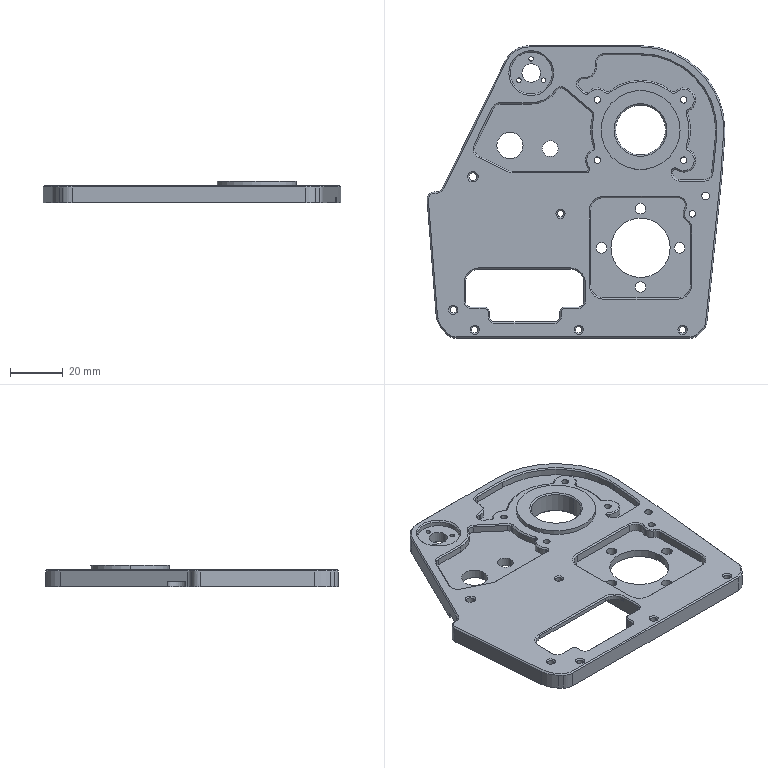Part | NX | features BREP 1 | 1 solid | 287 faces | box 113.03 x 111.071 x 8.2 mm | volume 44822 mm3 | cylinder 122 | plane 84 | cone 81 | commonest cylinder face diameters 2.5 x22 4 x20 6 x13 2 x12 10 x11 9 x7